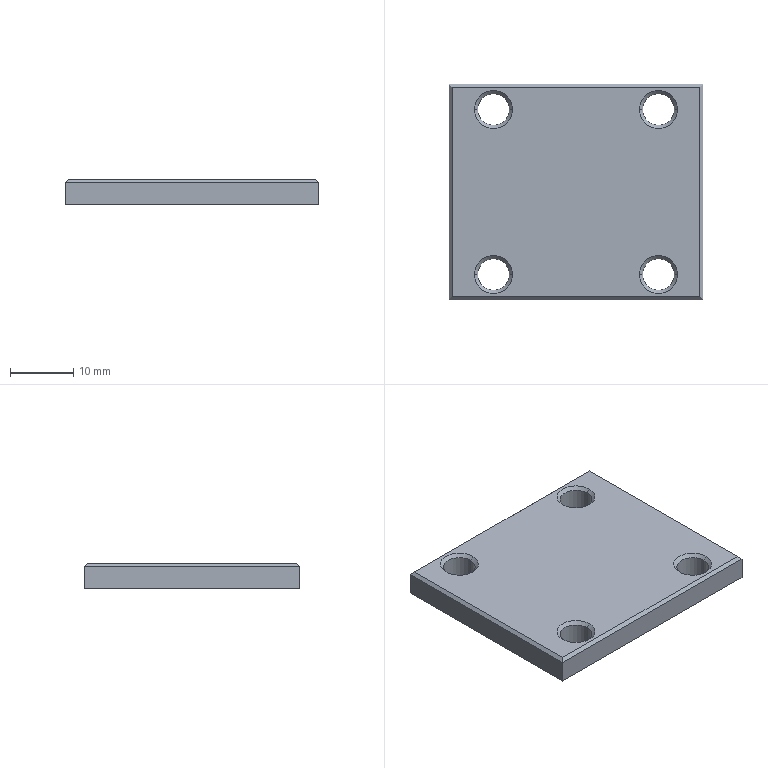Part | NX | 1 solid | 26 faces | box 40 x 34 x 4.05 mm | volume 5163 mm3 | plane 10 | cylinder 8 | cone 8 | commonest cylinder face diameters 5 x8
STEP:
#1=CARTESIAN_POINT('',(0.,0.,8.07));
#2=VERTEX_POINT('',#1);
#3=CARTESIAN_POINT('',(0.,-34.,8.07));
#4=VERTEX_POINT('',#3);
#5=CARTESIAN_POINT('',(0.,0.,8.07));
#6=DIRECTION('',(0.,-1.,0.));
#7=VECTOR('',#6,1000.);
#8=LINE('',#5,#7);
#9=EDGE_CURVE('',#2,#4,#8,.T.);
#10=ORIENTED_EDGE('',*,*,#9,.T.);
#11=CARTESIAN_POINT('',(0.5,-33.5,8.57));
#12=VERTEX_POINT('',#11);
#13=CARTESIAN_POINT('',(-8.07,-42.07,0.));
#14=DIRECTION('',(0.5774,0.5774,0.5774));
#15=VECTOR('',#14,1000.);
#16=LINE('',#13,#15);
#17=EDGE_CURVE('',#4,#12,#16,.T.);
#18=ORIENTED_EDGE('',*,*,#17,.T.);
#19=CARTESIAN_POINT('',(0.5,-0.5,8.57));
#20=VERTEX_POINT('',#19);
#21=CARTESIAN_POINT('',(0.5,0.,8.57));
#22=DIRECTION('',(0.,-1.,0.));
#23=VECTOR('',#22,1000.);
#24=LINE('',#21,#23);
#25=EDGE_CURVE('',#20,#12,#24,.T.);
#26=ORIENTED_EDGE('',*,*,#25,.F.);
#27=CARTESIAN_POINT('',(-8.07,8.07,0.));
#28=DIRECTION('',(0.5774,-0.5774,0.5774));
#29=VECTOR('',#28,1000.);
#30=LINE('',#27,#29);
#31=EDGE_CURVE('',#2,#20,#30,.T.);
#32=ORIENTED_EDGE('',*,*,#31,.F.);
#33=EDGE_LOOP('',(#10,#18,#26,#32));
#34=FACE_BOUND('',#33,.T.);
#35=CARTESIAN_POINT('',(0.25,-17.,8.32));
#36=DIRECTION('',(0.7071,0.,-0.7071));
#37=DIRECTION('',(0.,-1.,0.));
#38=AXIS2_PLACEMENT_3D('',#35,#36,#37);
#39=PLANE('',#38);
#40=ADVANCED_FACE('',(#34),#39,.F.);
#41=ORIENTED_EDGE('',*,*,#9,.F.);
#42=CARTESIAN_POINT('',(0.,0.,4.52));
#43=VERTEX_POINT('',#42);
#44=CARTESIAN_POINT('',(0.,0.,0.));
#45=DIRECTION('',(0.,0.,-1.));
#46=VECTOR('',#45,1000.);
#47=LINE('',#44,#46);
#48=EDGE_CURVE('',#2,#43,#47,.T.);
#49=ORIENTED_EDGE('',*,*,#48,.T.);
#50=CARTESIAN_POINT('',(0.,-34.,4.52));
#51=VERTEX_POINT('',#50);
#52=CARTESIAN_POINT('',(0.,0.,4.52));
#53=DIRECTION('',(0.,-1.,0.));
#54=VECTOR('',#53,1000.);
#55=LINE('',#52,#54);
#56=EDGE_CURVE('',#43,#51,#55,.T.);
#57=ORIENTED_EDGE('',*,*,#56,.T.);
#58=CARTESIAN_POINT('',(0.,-34.,0.));
#59=DIRECTION('',(0.,0.,1.));
#60=VECTOR('',#59,1000.);
#61=LINE('',#58,#60);
#62=EDGE_CURVE('',#51,#4,#61,.T.);
#63=ORIENTED_EDGE('',*,*,#62,.T.);
#64=EDGE_LOOP('',(#41,#49,#57,#63));
#65=FACE_BOUND('',#64,.T.);
#66=CARTESIAN_POINT('',(0.,0.,0.));
#67=DIRECTION('',(-1.,0.,0.));
#68=DIRECTION('',(0.,0.,1.));
#69=AXIS2_PLACEMENT_3D('',#66,#67,#68);
#70=PLANE('',#69);
#71=ADVANCED_FACE('',(#65),#70,.T.);
#72=CARTESIAN_POINT('',(40.,0.,8.07));
#73=VERTEX_POINT('',#72);
#74=CARTESIAN_POINT('',(0.,0.,8.07));
#75=DIRECTION('',(1.,0.,0.));
#76=VECTOR('',#75,1000.);
#77=LINE('',#74,#76);
#78=EDGE_CURVE('',#2,#73,#77,.T.);
#79=ORIENTED_EDGE('',*,*,#78,.T.);
#80=CARTESIAN_POINT('',(40.,0.,4.52));
#81=VERTEX_POINT('',#80);
#82=CARTESIAN_POINT('',(40.,0.,0.));
#83=DIRECTION('',(0.,0.,1.));
#84=VECTOR('',#83,1000.);
#85=LINE('',#82,#84);
#86=EDGE_CURVE('',#81,#73,#85,.T.);
#87=ORIENTED_EDGE('',*,*,#86,.F.);
#88=CARTESIAN_POINT('',(0.,0.,4.52));
#89=DIRECTION('',(-1.,0.,0.));
#90=VECTOR('',#89,1000.);
#91=LINE('',#88,#90);
#92=EDGE_CURVE('',#81,#43,#91,.T.);
#93=ORIENTED_EDGE('',*,*,#92,.T.);
#94=ORIENTED_EDGE('',*,*,#48,.F.);
#95=EDGE_LOOP('',(#79,#87,#93,#94));
#96=FACE_BOUND('',#95,.T.);
#97=CARTESIAN_POINT('',(40.,0.,0.));
#98=DIRECTION('',(0.,1.,0.));
#99=DIRECTION('',(1.,0.,0.));
#100=AXIS2_PLACEMENT_3D('',#97,#98,#99);
#101=PLANE('',#100);
#102=ADVANCED_FACE('',(#96),#101,.T.);
#103=CARTESIAN_POINT('',(40.,-34.,8.07));
#104=VERTEX_POINT('',#103);
#105=CARTESIAN_POINT('',(40.,0.,8.07));
#106=DIRECTION('',(0.,1.,0.));
#107=VECTOR('',#106,1000.);
#108=LINE('',#105,#107);
#109=EDGE_CURVE('',#104,#73,#108,.T.);
#110=ORIENTED_EDGE('',*,*,#109,.F.);
#111=CARTESIAN_POINT('',(40.,-34.,4.52));
#112=VERTEX_POINT('',#111);
#113=CARTESIAN_POINT('',(40.,-34.,0.));
#114=DIRECTION('',(0.,0.,-1.));
#115=VECTOR('',#114,1000.);
#116=LINE('',#113,#115);
#117=EDGE_CURVE('',#104,#112,#116,.T.);
#118=ORIENTED_EDGE('',*,*,#117,.T.);
#119=CARTESIAN_POINT('',(40.,0.,4.52));
#120=DIRECTION('',(0.,1.,0.));
#121=VECTOR('',#120,1000.);
#122=LINE('',#119,#121);
#123=EDGE_CURVE('',#112,#81,#122,.T.);
#124=ORIENTED_EDGE('',*,*,#123,.T.);
#125=ORIENTED_EDGE('',*,*,#86,.T.);
#126=EDGE_LOOP('',(#110,#118,#124,#125));
#127=FACE_BOUND('',#126,.T.);
#128=CARTESIAN_POINT('',(40.,-34.,0.));
#129=DIRECTION('',(1.,0.,0.));
#130=DIRECTION('',(0.,1.,0.));
#131=AXIS2_PLACEMENT_3D('',#128,#129,#130);
#132=PLANE('',#131);
#133=ADVANCED_FACE('',(#127),#132,.T.);
#134=CARTESIAN_POINT('',(0.,-34.,8.07));
#135=DIRECTION('',(1.,0.,0.));
#136=VECTOR('',#135,1000.);
#137=LINE('',#134,#136);
#138=EDGE_CURVE('',#4,#104,#137,.T.);
#139=ORIENTED_EDGE('',*,*,#138,.F.);
#140=ORIENTED_EDGE('',*,*,#62,.F.);
#141=CARTESIAN_POINT('',(0.,-34.,4.52));
#142=DIRECTION('',(1.,0.,0.));
#143=VECTOR('',#142,1000.);
#144=LINE('',#141,#143);
#145=EDGE_CURVE('',#51,#112,#144,.T.);
#146=ORIENTED_EDGE('',*,*,#145,.T.);
#147=ORIENTED_EDGE('',*,*,#117,.F.);
#148=EDGE_LOOP('',(#139,#140,#146,#147));
#149=FACE_BOUND('',#148,.T.);
#150=CARTESIAN_POINT('',(0.,-34.,0.));
#151=DIRECTION('',(0.,-1.,0.));
#152=DIRECTION('',(0.,0.,-1.));
#153=AXIS2_PLACEMENT_3D('',#150,#151,#152);
#154=PLANE('',#153);
#155=ADVANCED_FACE('',(#149),#154,.T.);
#156=ORIENTED_EDGE('',*,*,#92,.F.);
#157=ORIENTED_EDGE('',*,*,#123,.F.);
#158=ORIENTED_EDGE('',*,*,#145,.F.);
#159=ORIENTED_EDGE('',*,*,#56,.F.);
#160=EDGE_LOOP('',(#156,#157,#158,#159));
#161=FACE_BOUND('',#160,.T.);
#162=CARTESIAN_POINT('',(4.5,-30.,4.52));
#163=VERTEX_POINT('',#162);
#164=CARTESIAN_POINT('',(9.5,-30.,4.52));
#165=VERTEX_POINT('',#164);
#166=CARTESIAN_POINT('',(7.,-30.,4.52));
#167=DIRECTION('',(0.,0.,-1.));
#168=DIRECTION('',(-1.,0.,0.));
#169=AXIS2_PLACEMENT_3D('',#166,#167,#168);
#170=CIRCLE('',#169,2.5);
#171=EDGE_CURVE('',#163,#165,#170,.T.);
#172=ORIENTED_EDGE('',*,*,#171,.F.);
#173=CARTESIAN_POINT('',(7.,-30.,4.52));
#174=DIRECTION('',(0.,0.,-1.));
#175=DIRECTION('',(-1.,0.,0.));
#176=AXIS2_PLACEMENT_3D('',#173,#174,#175);
#177=CIRCLE('',#176,2.5);
#178=EDGE_CURVE('',#165,#163,#177,.T.);
#179=ORIENTED_EDGE('',*,*,#178,.F.);
#180=EDGE_LOOP('',(#172,#179));
#181=FACE_BOUND('',#180,.T.);
#182=CARTESIAN_POINT('',(4.5,-4.,4.52));
#183=VERTEX_POINT('',#182);
#184=CARTESIAN_POINT('',(9.5,-4.,4.52));
#185=VERTEX_POINT('',#184);
#186=CARTESIAN_POINT('',(7.,-4.,4.52));
#187=DIRECTION('',(0.,0.,-1.));
#188=DIRECTION('',(-1.,0.,0.));
#189=AXIS2_PLACEMENT_3D('',#186,#187,#188);
#190=CIRCLE('',#189,2.5);
#191=EDGE_CURVE('',#183,#185,#190,.T.);
#192=ORIENTED_EDGE('',*,*,#191,.F.);
#193=CARTESIAN_POINT('',(7.,-4.,4.52));
#194=DIRECTION('',(0.,0.,-1.));
#195=DIRECTION('',(-1.,0.,0.));
#196=AXIS2_PLACEMENT_3D('',#193,#194,#195);
#197=CIRCLE('',#196,2.5);
#198=EDGE_CURVE('',#185,#183,#197,.T.);
#199=ORIENTED_EDGE('',*,*,#198,.F.);
#200=EDGE_LOOP('',(#192,#199));
#201=FACE_BOUND('',#200,.T.);
#202=CARTESIAN_POINT('',(30.5,-4.,4.52));
#203=VERTEX_POINT('',#202);
#204=CARTESIAN_POINT('',(35.5,-4.,4.52));
#205=VERTEX_POINT('',#204);
#206=CARTESIAN_POINT('',(33.,-4.,4.52));
#207=DIRECTION('',(0.,0.,-1.));
#208=DIRECTION('',(-1.,0.,0.));
#209=AXIS2_PLACEMENT_3D('',#206,#207,#208);
#210=CIRCLE('',#209,2.5);
#211=EDGE_CURVE('',#203,#205,#210,.T.);
#212=ORIENTED_EDGE('',*,*,#211,.F.);
#213=CARTESIAN_POINT('',(33.,-4.,4.52));
#214=DIRECTION('',(0.,0.,-1.));
#215=DIRECTION('',(-1.,0.,0.));
#216=AXIS2_PLACEMENT_3D('',#213,#214,#215);
#217=CIRCLE('',#216,2.5);
#218=EDGE_CURVE('',#205,#203,#217,.T.);
#219=ORIENTED_EDGE('',*,*,#218,.F.);
#220=EDGE_LOOP('',(#212,#219));
#221=FACE_BOUND('',#220,.T.);
#222=CARTESIAN_POINT('',(30.5,-30.,4.52));
#223=VERTEX_POINT('',#222);
#224=CARTESIAN_POINT('',(35.5,-30.,4.52));
#225=VERTEX_POINT('',#224);
#226=CARTESIAN_POINT('',(33.,-30.,4.52));
#227=DIRECTION('',(0.,0.,-1.));
#228=DIRECTION('',(-1.,0.,0.));
#229=AXIS2_PLACEMENT_3D('',#226,#227,#228);
#230=CIRCLE('',#229,2.5);
#231=EDGE_CURVE('',#223,#225,#230,.T.);
#232=ORIENTED_EDGE('',*,*,#231,.F.);
#233=CARTESIAN_POINT('',(33.,-30.,4.52));
#234=DIRECTION('',(0.,0.,-1.));
#235=DIRECTION('',(-1.,0.,0.));
#236=AXIS2_PLACEMENT_3D('',#233,#234,#235);
#237=CIRCLE('',#236,2.5);
#238=EDGE_CURVE('',#225,#223,#237,.T.);
#239=ORIENTED_EDGE('',*,*,#238,.F.);
#240=EDGE_LOOP('',(#232,#239));
#241=FACE_BOUND('',#240,.T.);
#242=CARTESIAN_POINT('',(-167.,62.,4.52));
#243=DIRECTION('',(0.,0.,1.));
#244=DIRECTION('',(1.,0.,0.));
#245=AXIS2_PLACEMENT_3D('',#242,#243,#244);
#246=PLANE('',#245);
#247=ADVANCED_FACE('',(#161,#181,#201,#221,#241),#246,.F.);
#248=CARTESIAN_POINT('',(9.5,-4.,8.07));
#249=VERTEX_POINT('',#248);
#250=CARTESIAN_POINT('',(4.5,-4.,8.07));
#251=VERTEX_POINT('',#250);
#252=CARTESIAN_POINT('',(7.,-4.,8.07));
#253=DIRECTION('',(0.,0.,-1.));
#254=DIRECTION('',(-1.,0.,0.));
#255=AXIS2_PLACEMENT_3D('',#252,#253,#254);
#256=CIRCLE('',#255,2.5);
#257=EDGE_CURVE('',#249,#251,#256,.T.);
#258=ORIENTED_EDGE('',*,*,#257,.F.);
#259=CARTESIAN_POINT('',(9.5,-4.,10.5));
#260=DIRECTION('',(0.,0.,-1.));
#261=VECTOR('',#260,1000.);
#262=LINE('',#259,#261);
#263=EDGE_CURVE('',#249,#185,#262,.T.);
#264=ORIENTED_EDGE('',*,*,#263,.T.);
#265=ORIENTED_EDGE('',*,*,#198,.T.);
#266=CARTESIAN_POINT('',(4.5,-4.,10.5));
#267=DIRECTION('',(0.,0.,-1.));
#268=VECTOR('',#267,1000.);
#269=LINE('',#266,#268);
#270=EDGE_CURVE('',#251,#183,#269,.T.);
#271=ORIENTED_EDGE('',*,*,#270,.F.);
#272=EDGE_LOOP('',(#258,#264,#265,#271));
#273=FACE_BOUND('',#272,.T.);
#274=CARTESIAN_POINT('',(7.,-4.,10.5));
#275=DIRECTION('',(0.,0.,-1.));
#276=DIRECTION('',(-1.,0.,0.));
#277=AXIS2_PLACEMENT_3D('',#274,#275,#276);
#278=CYLINDRICAL_SURFACE('',#277,2.5);
#279=ADVANCED_FACE('',(#273),#278,.F.);
#280=CARTESIAN_POINT('',(35.5,-4.,8.07));
#281=VERTEX_POINT('',#280);
#282=CARTESIAN_POINT('',(30.5,-4.,8.07));
#283=VERTEX_POINT('',#282);
#284=CARTESIAN_POINT('',(33.,-4.,8.07));
#285=DIRECTION('',(0.,0.,1.));
#286=DIRECTION('',(1.,0.,0.));
#287=AXIS2_PLACEMENT_3D('',#284,#285,#286);
#288=CIRCLE('',#287,2.5);
#289=EDGE_CURVE('',#281,#283,#288,.T.);
#290=ORIENTED_EDGE('',*,*,#289,.T.);
#291=CARTESIAN_POINT('',(30.5,-4.,10.5));
#292=DIRECTION('',(0.,0.,-1.));
#293=VECTOR('',#292,1000.);
#294=LINE('',#291,#293);
#295=EDGE_CURVE('',#203,#283,#294,.F.);
#296=ORIENTED_EDGE('',*,*,#295,.F.);
#297=ORIENTED_EDGE('',*,*,#211,.T.);
#298=CARTESIAN_POINT('',(35.5,-4.,10.5));
#299=DIRECTION('',(0.,0.,-1.));
#300=VECTOR('',#299,1000.);
#301=LINE('',#298,#300);
#302=EDGE_CURVE('',#205,#281,#301,.F.);
#303=ORIENTED_EDGE('',*,*,#302,.T.);
#304=EDGE_LOOP('',(#290,#296,#297,#303));
#305=FACE_BOUND('',#304,.T.);
#306=CARTESIAN_POINT('',(33.,-4.,10.5));
#307=DIRECTION('',(0.,0.,-1.));
#308=DIRECTION('',(-1.,0.,0.));
#309=AXIS2_PLACEMENT_3D('',#306,#307,#308);
#310=CYLINDRICAL_SURFACE('',#309,2.5);
#311=ADVANCED_FACE('',(#305),#310,.F.);
#312=ORIENTED_EDGE('',*,*,#171,.T.);
#313=CARTESIAN_POINT('',(9.5,-30.,8.07));
#314=VERTEX_POINT('',#313);
#315=CARTESIAN_POINT('',(9.5,-30.,10.5));
#316=DIRECTION('',(0.,0.,-1.));
#317=VECTOR('',#316,1000.);
#318=LINE('',#315,#317);
#319=EDGE_CURVE('',#314,#165,#318,.T.);
#320=ORIENTED_EDGE('',*,*,#319,.F.);
#321=CARTESIAN_POINT('',(4.5,-30.,8.07));
#322=VERTEX_POINT('',#321);
#323=CARTESIAN_POINT('',(7.,-30.,8.07));
#324=DIRECTION('',(0.,0.,1.));
#325=DIRECTION('',(1.,0.,0.));
#326=AXIS2_PLACEMENT_3D('',#323,#324,#325);
#327=CIRCLE('',#326,2.5);
#328=EDGE_CURVE('',#314,#322,#327,.T.);
#329=ORIENTED_EDGE('',*,*,#328,.T.);
#330=CARTESIAN_POINT('',(4.5,-30.,10.5));
#331=DIRECTION('',(0.,0.,-1.));
#332=VECTOR('',#331,1000.);
#333=LINE('',#330,#332);
#334=EDGE_CURVE('',#322,#163,#333,.T.);
#335=ORIENTED_EDGE('',*,*,#334,.T.);
#336=EDGE_LOOP('',(#312,#320,#329,#335));
#337=FACE_BOUND('',#336,.T.);
#338=CARTESIAN_POINT('',(7.,-30.,10.5));
#339=DIRECTION('',(0.,0.,-1.));
#340=DIRECTION('',(-1.,0.,0.));
#341=AXIS2_PLACEMENT_3D('',#338,#339,#340);
#342=CYLINDRICAL_SURFACE('',#341,2.5);
#343=ADVANCED_FACE('',(#337),#342,.F.);
#344=ORIENTED_EDGE('',*,*,#231,.T.);
#345=CARTESIAN_POINT('',(35.5,-30.,8.07));
#346=VERTEX_POINT('',#345);
#347=CARTESIAN_POINT('',(35.5,-30.,10.5));
#348=DIRECTION('',(0.,0.,-1.));
#349=VECTOR('',#348,1000.);
#350=LINE('',#347,#349);
#351=EDGE_CURVE('',#346,#225,#350,.T.);
#352=ORIENTED_EDGE('',*,*,#351,.F.);
#353=CARTESIAN_POINT('',(30.5,-30.,8.07));
#354=VERTEX_POINT('',#353);
#355=CARTESIAN_POINT('',(33.,-30.,8.07));
#356=DIRECTION('',(0.,0.,-1.));
#357=DIRECTION('',(-1.,0.,0.));
#358=AXIS2_PLACEMENT_3D('',#355,#356,#357);
#359=CIRCLE('',#358,2.5);
#360=EDGE_CURVE('',#354,#346,#359,.T.);
#361=ORIENTED_EDGE('',*,*,#360,.F.);
#362=CARTESIAN_POINT('',(30.5,-30.,10.5));
#363=DIRECTION('',(0.,0.,-1.));
#364=VECTOR('',#363,1000.);
#365=LINE('',#362,#364);
#366=EDGE_CURVE('',#354,#223,#365,.T.);
#367=ORIENTED_EDGE('',*,*,#366,.T.);
#368=EDGE_LOOP('',(#344,#352,#361,#367));
#369=FACE_BOUND('',#368,.T.);
#370=CARTESIAN_POINT('',(33.,-30.,10.5));
#371=DIRECTION('',(0.,0.,-1.));
#372=DIRECTION('',(-1.,0.,0.));
#373=AXIS2_PLACEMENT_3D('',#370,#371,#372);
#374=CYLINDRICAL_SURFACE('',#373,2.5);
#375=ADVANCED_FACE('',(#369),#374,.F.);
#376=ORIENTED_EDGE('',*,*,#257,.T.);
#377=CARTESIAN_POINT('',(4.,-4.,8.57));
#378=VERTEX_POINT('',#377);
#379=CARTESIAN_POINT('',(4.,-4.,8.57));
#380=DIRECTION('',(-0.7071,0.,0.7071));
#381=VECTOR('',#380,1000.);
#382=LINE('',#379,#381);
#383=EDGE_CURVE('',#378,#251,#382,.F.);
#384=ORIENTED_EDGE('',*,*,#383,.F.);
#385=CARTESIAN_POINT('',(10.,-4.,8.57));
#386=VERTEX_POINT('',#385);
#387=CARTESIAN_POINT('',(7.,-4.,8.57));
#388=DIRECTION('',(0.,0.,1.));
#389=DIRECTION('',(1.,0.,0.));
#390=AXIS2_PLACEMENT_3D('',#387,#388,#389);
#391=CIRCLE('',#390,3.);
#392=EDGE_CURVE('',#378,#386,#391,.T.);
#393=ORIENTED_EDGE('',*,*,#392,.T.);
#394=CARTESIAN_POINT('',(10.,-4.,8.57));
#395=DIRECTION('',(0.7071,0.,0.7071));
#396=VECTOR('',#395,1000.);
#397=LINE('',#394,#396);
#398=EDGE_CURVE('',#386,#249,#397,.F.);
#399=ORIENTED_EDGE('',*,*,#398,.T.);
#400=EDGE_LOOP('',(#376,#384,#393,#399));
#401=FACE_BOUND('',#400,.T.);
#402=CARTESIAN_POINT('',(7.,-4.,8.57));
#403=DIRECTION('',(0.,0.,1.));
#404=DIRECTION('',(1.,0.,0.));
#405=AXIS2_PLACEMENT_3D('',#402,#403,#404);
#406=CONICAL_SURFACE('',#405,3.,0.7854);
#407=ADVANCED_FACE('',(#401),#406,.F.);
#408=CARTESIAN_POINT('',(7.,-30.,8.07));
#409=DIRECTION('',(0.,0.,1.));
#410=DIRECTION('',(1.,0.,0.));
#411=AXIS2_PLACEMENT_3D('',#408,#409,#410);
#412=CIRCLE('',#411,2.5);
#413=EDGE_CURVE('',#322,#314,#412,.T.);
#414=ORIENTED_EDGE('',*,*,#413,.F.);
#415=CARTESIAN_POINT('',(4.,-30.,8.57));
#416=VERTEX_POINT('',#415);
#417=CARTESIAN_POINT('',(4.,-30.,8.57));
#418=DIRECTION('',(-0.7071,0.,0.7071));
#419=VECTOR('',#418,1000.);
#420=LINE('',#417,#419);
#421=EDGE_CURVE('',#322,#416,#420,.T.);
#422=ORIENTED_EDGE('',*,*,#421,.T.);
#423=CARTESIAN_POINT('',(10.,-30.,8.57));
#424=VERTEX_POINT('',#423);
#425=CARTESIAN_POINT('',(7.,-30.,8.57));
#426=DIRECTION('',(0.,0.,1.));
#427=DIRECTION('',(1.,0.,0.));
#428=AXIS2_PLACEMENT_3D('',#425,#426,#427);
#429=CIRCLE('',#428,3.);
#430=EDGE_CURVE('',#416,#424,#429,.T.);
#431=ORIENTED_EDGE('',*,*,#430,.T.);
#432=CARTESIAN_POINT('',(10.,-30.,8.57));
#433=DIRECTION('',(0.7071,0.,0.7071));
#434=VECTOR('',#433,1000.);
#435=LINE('',#432,#434);
#436=EDGE_CURVE('',#314,#424,#435,.T.);
#437=ORIENTED_EDGE('',*,*,#436,.F.);
#438=EDGE_LOOP('',(#414,#422,#431,#437));
#439=FACE_BOUND('',#438,.T.);
#440=CARTESIAN_POINT('',(7.,-30.,8.57));
#441=DIRECTION('',(0.,0.,1.));
#442=DIRECTION('',(1.,0.,0.));
#443=AXIS2_PLACEMENT_3D('',#440,#441,#442);
#444=CONICAL_SURFACE('',#443,3.,0.7854);
#445=ADVANCED_FACE('',(#439),#444,.F.);
#446=CARTESIAN_POINT('',(30.,-30.,8.57));
#447=VERTEX_POINT('',#446);
#448=CARTESIAN_POINT('',(36.,-30.,8.57));
#449=VERTEX_POINT('',#448);
#450=CARTESIAN_POINT('',(33.,-30.,8.57));
#451=DIRECTION('',(0.,0.,1.));
#452=DIRECTION('',(1.,0.,0.));
#453=AXIS2_PLACEMENT_3D('',#450,#451,#452);
#454=CIRCLE('',#453,3.);
#455=EDGE_CURVE('',#447,#449,#454,.T.);
#456=ORIENTED_EDGE('',*,*,#455,.T.);
#457=CARTESIAN_POINT('',(36.,-30.,8.57));
#458=DIRECTION('',(0.7071,0.,0.7071));
#459=VECTOR('',#458,1000.);
#460=LINE('',#457,#459);
#461=EDGE_CURVE('',#346,#449,#460,.T.);
#462=ORIENTED_EDGE('',*,*,#461,.F.);
#463=CARTESIAN_POINT('',(33.,-30.,8.07));
#464=DIRECTION('',(0.,0.,-1.));
#465=DIRECTION('',(-1.,0.,0.));
#466=AXIS2_PLACEMENT_3D('',#463,#464,#465);
#467=CIRCLE('',#466,2.5);
#468=EDGE_CURVE('',#346,#354,#467,.T.);
#469=ORIENTED_EDGE('',*,*,#468,.T.);
#470=CARTESIAN_POINT('',(30.,-30.,8.57));
#471=DIRECTION('',(-0.7071,0.,0.7071));
#472=VECTOR('',#471,1000.);
#473=LINE('',#470,#472);
#474=EDGE_CURVE('',#354,#447,#473,.T.);
#475=ORIENTED_EDGE('',*,*,#474,.T.);
#476=EDGE_LOOP('',(#456,#462,#469,#475));
#477=FACE_BOUND('',#476,.T.);
#478=CARTESIAN_POINT('',(33.,-30.,8.57));
#479=DIRECTION('',(0.,0.,1.));
#480=DIRECTION('',(1.,0.,0.));
#481=AXIS2_PLACEMENT_3D('',#478,#479,#480);
#482=CONICAL_SURFACE('',#481,3.,0.7854);
#483=ADVANCED_FACE('',(#477),#482,.F.);
#484=CARTESIAN_POINT('',(36.,-4.,8.57));
#485=VERTEX_POINT('',#484);
#486=CARTESIAN_POINT('',(30.,-4.,8.57));
#487=VERTEX_POINT('',#486);
#488=CARTESIAN_POINT('',(33.,-4.,8.57));
#489=DIRECTION('',(0.,0.,1.));
#490=DIRECTION('',(1.,0.,0.));
#491=AXIS2_PLACEMENT_3D('',#488,#489,#490);
#492=CIRCLE('',#491,3.);
#493=EDGE_CURVE('',#485,#487,#492,.T.);
#494=ORIENTED_EDGE('',*,*,#493,.T.);
#495=CARTESIAN_POINT('',(30.,-4.,8.57));
#496=DIRECTION('',(-0.7071,0.,0.7071));
#497=VECTOR('',#496,1000.);
#498=LINE('',#495,#497);
#499=EDGE_CURVE('',#283,#487,#498,.T.);
#500=ORIENTED_EDGE('',*,*,#499,.F.);
#501=ORIENTED_EDGE('',*,*,#289,.F.);
#502=CARTESIAN_POINT('',(36.,-4.,8.57));
#503=DIRECTION('',(0.7071,0.,0.7071));
#504=VECTOR('',#503,1000.);
#505=LINE('',#502,#504);
#506=EDGE_CURVE('',#281,#485,#505,.T.);
#507=ORIENTED_EDGE('',*,*,#506,.T.);
#508=EDGE_LOOP('',(#494,#500,#501,#507));
#509=FACE_BOUND('',#508,.T.);
#510=CARTESIAN_POINT('',(33.,-4.,8.57));
#511=DIRECTION('',(0.,0.,1.));
#512=DIRECTION('',(1.,0.,0.));
#513=AXIS2_PLACEMENT_3D('',#510,#511,#512);
#514=CONICAL_SURFACE('',#513,3.,0.7854);
#515=ADVANCED_FACE('',(#509),#514,.F.);
#516=ORIENTED_EDGE('',*,*,#138,.T.);
#517=CARTESIAN_POINT('',(39.5,-33.5,8.57));
#518=VERTEX_POINT('',#517);
#519=CARTESIAN_POINT('',(48.07,-42.07,0.));
#520=DIRECTION('',(-0.5774,0.5774,0.5774));
#521=VECTOR('',#520,1000.);
#522=LINE('',#519,#521);
#523=EDGE_CURVE('',#104,#518,#522,.T.);
#524=ORIENTED_EDGE('',*,*,#523,.T.);
#525=CARTESIAN_POINT('',(0.,-33.5,8.57));
#526=DIRECTION('',(1.,0.,0.));
#527=VECTOR('',#526,1000.);
#528=LINE('',#525,#527);
#529=EDGE_CURVE('',#12,#518,#528,.T.);
#530=ORIENTED_EDGE('',*,*,#529,.F.);
#531=ORIENTED_EDGE('',*,*,#17,.F.);
#532=EDGE_LOOP('',(#516,#524,#530,#531));
#533=FACE_BOUND('',#532,.T.);
#534=CARTESIAN_POINT('',(20.,-33.75,8.32));
#535=DIRECTION('',(0.,0.7071,-0.7071));
#536=DIRECTION('',(-1.,0.,0.));
#537=AXIS2_PLACEMENT_3D('',#534,#535,#536);
#538=PLANE('',#537);
#539=ADVANCED_FACE('',(#533),#538,.F.);
#540=ORIENTED_EDGE('',*,*,#109,.T.);
#541=CARTESIAN_POINT('',(39.5,-0.5,8.57));
#542=VERTEX_POINT('',#541);
#543=CARTESIAN_POINT('',(48.07,8.07,0.));
#544=DIRECTION('',(-0.5774,-0.5774,0.5774));
#545=VECTOR('',#544,1000.);
#546=LINE('',#543,#545);
#547=EDGE_CURVE('',#73,#542,#546,.T.);
#548=ORIENTED_EDGE('',*,*,#547,.T.);
#549=CARTESIAN_POINT('',(39.5,0.,8.57));
#550=DIRECTION('',(0.,-1.,0.));
#551=VECTOR('',#550,1000.);
#552=LINE('',#549,#551);
#553=EDGE_CURVE('',#542,#518,#552,.T.);
#554=ORIENTED_EDGE('',*,*,#553,.T.);
#555=ORIENTED_EDGE('',*,*,#523,.F.);
#556=EDGE_LOOP('',(#540,#548,#554,#555));
#557=FACE_BOUND('',#556,.T.);
#558=CARTESIAN_POINT('',(39.75,-17.,8.32));
#559=DIRECTION('',(0.7071,0.,0.7071));
#560=DIRECTION('',(0.,-1.,0.));
#561=AXIS2_PLACEMENT_3D('',#558,#559,#560);
#562=PLANE('',#561);
#563=ADVANCED_FACE('',(#557),#562,.T.);
#564=ORIENTED_EDGE('',*,*,#78,.F.);
#565=ORIENTED_EDGE('',*,*,#31,.T.);
#566=CARTESIAN_POINT('',(0.,-0.5,8.57));
#567=DIRECTION('',(1.,0.,0.));
#568=VECTOR('',#567,1000.);
#569=LINE('',#566,#568);
#570=EDGE_CURVE('',#20,#542,#569,.T.);
#571=ORIENTED_EDGE('',*,*,#570,.T.);
#572=ORIENTED_EDGE('',*,*,#547,.F.);
#573=EDGE_LOOP('',(#564,#565,#571,#572));
#574=FACE_BOUND('',#573,.T.);
#575=CARTESIAN_POINT('',(20.,-0.25,8.32));
#576=DIRECTION('',(0.,0.7071,0.7071));
#577=DIRECTION('',(1.,0.,0.));
#578=AXIS2_PLACEMENT_3D('',#575,#576,#577);
#579=PLANE('',#578);
#580=ADVANCED_FACE('',(#574),#579,.T.);
#581=ORIENTED_EDGE('',*,*,#25,.T.);
#582=ORIENTED_EDGE('',*,*,#529,.T.);
#583=ORIENTED_EDGE('',*,*,#553,.F.);
#584=ORIENTED_EDGE('',*,*,#570,.F.);
#585=EDGE_LOOP('',(#581,#582,#583,#584));
#586=FACE_BOUND('',#585,.T.);
#587=CARTESIAN_POINT('',(7.,-4.,8.57));
#588=DIRECTION('',(0.,0.,1.));
#589=DIRECTION('',(1.,0.,0.));
#590=AXIS2_PLACEMENT_3D('',#587,#588,#589);
#591=CIRCLE('',#590,3.);
#592=EDGE_CURVE('',#386,#378,#591,.T.);
#593=ORIENTED_EDGE('',*,*,#592,.F.);
#594=ORIENTED_EDGE('',*,*,#392,.F.);
#595=EDGE_LOOP('',(#593,#594));
#596=FACE_BOUND('',#595,.T.);
#597=ORIENTED_EDGE('',*,*,#455,.F.);
#598=CARTESIAN_POINT('',(33.,-30.,8.57));
#599=DIRECTION('',(0.,0.,1.));
#600=DIRECTION('',(1.,0.,0.));
#601=AXIS2_PLACEMENT_3D('',#598,#599,#600);
#602=CIRCLE('',#601,3.);
#603=EDGE_CURVE('',#449,#447,#602,.T.);
#604=ORIENTED_EDGE('',*,*,#603,.F.);
#605=EDGE_LOOP('',(#597,#604));
#606=FACE_BOUND('',#605,.T.);
#607=ORIENTED_EDGE('',*,*,#493,.F.);
#608=CARTESIAN_POINT('',(33.,-4.,8.57));
#609=DIRECTION('',(0.,0.,1.));
#610=DIRECTION('',(1.,0.,0.));
#611=AXIS2_PLACEMENT_3D('',#608,#609,#610);
#612=CIRCLE('',#611,3.);
#613=EDGE_CURVE('',#487,#485,#612,.T.);
#614=ORIENTED_EDGE('',*,*,#613,.F.);
#615=EDGE_LOOP('',(#607,#614));
#616=FACE_BOUND('',#615,.T.);
#617=ORIENTED_EDGE('',*,*,#430,.F.);
#618=CARTESIAN_POINT('',(7.,-30.,8.57));
#619=DIRECTION('',(0.,0.,1.));
#620=DIRECTION('',(1.,0.,0.));
#621=AXIS2_PLACEMENT_3D('',#618,#619,#620);
#622=CIRCLE('',#621,3.);
#623=EDGE_CURVE('',#424,#416,#622,.T.);
#624=ORIENTED_EDGE('',*,*,#623,.F.);
#625=EDGE_LOOP('',(#617,#624));
#626=FACE_BOUND('',#625,.T.);
#627=CARTESIAN_POINT('',(0.,0.,8.57));
#628=DIRECTION('',(0.,0.,1.));
#629=DIRECTION('',(1.,0.,0.));
#630=AXIS2_PLACEMENT_3D('',#627,#628,#629);
#631=PLANE('',#630);
#632=ADVANCED_FACE('',(#586,#596,#606,#616,#626),#631,.T.);
#633=ORIENTED_EDGE('',*,*,#461,.T.);
#634=ORIENTED_EDGE('',*,*,#603,.T.);
#635=ORIENTED_EDGE('',*,*,#474,.F.);
#636=ORIENTED_EDGE('',*,*,#360,.T.);
#637=EDGE_LOOP('',(#633,#634,#635,#636));
#638=FACE_BOUND('',#637,.T.);
#639=CARTESIAN_POINT('',(33.,-30.,8.57));
#640=DIRECTION('',(0.,0.,1.));
#641=DIRECTION('',(1.,0.,0.));
#642=AXIS2_PLACEMENT_3D('',#639,#640,#641);
#643=CONICAL_SURFACE('',#642,3.,0.7854);
#644=ADVANCED_FACE('',(#638),#643,.F.);
#645=ORIENTED_EDGE('',*,*,#295,.T.);
#646=CARTESIAN_POINT('',(33.,-4.,8.07));
#647=DIRECTION('',(0.,0.,1.));
#648=DIRECTION('',(1.,0.,0.));
#649=AXIS2_PLACEMENT_3D('',#646,#647,#648);
#650=CIRCLE('',#649,2.5);
#651=EDGE_CURVE('',#283,#281,#650,.T.);
#652=ORIENTED_EDGE('',*,*,#651,.T.);
#653=ORIENTED_EDGE('',*,*,#302,.F.);
#654=ORIENTED_EDGE('',*,*,#218,.T.);
#655=EDGE_LOOP('',(#645,#652,#653,#654));
#656=FACE_BOUND('',#655,.T.);
#657=CARTESIAN_POINT('',(33.,-4.,10.5));
#658=DIRECTION('',(0.,0.,-1.));
#659=DIRECTION('',(-1.,0.,0.));
#660=AXIS2_PLACEMENT_3D('',#657,#658,#659);
#661=CYLINDRICAL_SURFACE('',#660,2.5);
#662=ADVANCED_FACE('',(#656),#661,.F.);
#663=ORIENTED_EDGE('',*,*,#506,.F.);
#664=ORIENTED_EDGE('',*,*,#651,.F.);
#665=ORIENTED_EDGE('',*,*,#499,.T.);
#666=ORIENTED_EDGE('',*,*,#613,.T.);
#667=EDGE_LOOP('',(#663,#664,#665,#666));
#668=FACE_BOUND('',#667,.T.);
#669=CARTESIAN_POINT('',(33.,-4.,8.57));
#670=DIRECTION('',(0.,0.,1.));
#671=DIRECTION('',(1.,0.,0.));
#672=AXIS2_PLACEMENT_3D('',#669,#670,#671);
#673=CONICAL_SURFACE('',#672,3.,0.7854);
#674=ADVANCED_FACE('',(#668),#673,.F.);
#675=ORIENTED_EDGE('',*,*,#413,.T.);
#676=ORIENTED_EDGE('',*,*,#319,.T.);
#677=ORIENTED_EDGE('',*,*,#178,.T.);
#678=ORIENTED_EDGE('',*,*,#334,.F.);
#679=EDGE_LOOP('',(#675,#676,#677,#678));
#680=FACE_BOUND('',#679,.T.);
#681=CARTESIAN_POINT('',(7.,-30.,10.5));
#682=DIRECTION('',(0.,0.,-1.));
#683=DIRECTION('',(-1.,0.,0.));
#684=AXIS2_PLACEMENT_3D('',#681,#682,#683);
#685=CYLINDRICAL_SURFACE('',#684,2.5);
#686=ADVANCED_FACE('',(#680),#685,.F.);
#687=ORIENTED_EDGE('',*,*,#592,.T.);
#688=ORIENTED_EDGE('',*,*,#383,.T.);
#689=CARTESIAN_POINT('',(7.,-4.,8.07));
#690=DIRECTION('',(0.,0.,-1.));
#691=DIRECTION('',(-1.,0.,0.));
#692=AXIS2_PLACEMENT_3D('',#689,#690,#691);
#693=CIRCLE('',#692,2.5);
#694=EDGE_CURVE('',#251,#249,#693,.T.);
#695=ORIENTED_EDGE('',*,*,#694,.T.);
#696=ORIENTED_EDGE('',*,*,#398,.F.);
#697=EDGE_LOOP('',(#687,#688,#695,#696));
#698=FACE_BOUND('',#697,.T.);
#699=CARTESIAN_POINT('',(7.,-4.,8.57));
#700=DIRECTION('',(0.,0.,1.));
#701=DIRECTION('',(1.,0.,0.));
#702=AXIS2_PLACEMENT_3D('',#699,#700,#701);
#703=CONICAL_SURFACE('',#702,3.,0.7854);
#704=ADVANCED_FACE('',(#698),#703,.F.);
#705=ORIENTED_EDGE('',*,*,#468,.F.);
#706=ORIENTED_EDGE('',*,*,#351,.T.);
#707=ORIENTED_EDGE('',*,*,#238,.T.);
#708=ORIENTED_EDGE('',*,*,#366,.F.);
#709=EDGE_LOOP('',(#705,#706,#707,#708));
#710=FACE_BOUND('',#709,.T.);
#711=CARTESIAN_POINT('',(33.,-30.,10.5));
#712=DIRECTION('',(0.,0.,-1.));
#713=DIRECTION('',(-1.,0.,0.));
#714=AXIS2_PLACEMENT_3D('',#711,#712,#713);
#715=CYLINDRICAL_SURFACE('',#714,2.5);
#716=ADVANCED_FACE('',(#710),#715,.F.);
#717=ORIENTED_EDGE('',*,*,#436,.T.);
#718=ORIENTED_EDGE('',*,*,#623,.T.);
#719=ORIENTED_EDGE('',*,*,#421,.F.);
#720=ORIENTED_EDGE('',*,*,#328,.F.);
#721=EDGE_LOOP('',(#717,#718,#719,#720));
#722=FACE_BOUND('',#721,.T.);
#723=CARTESIAN_POINT('',(7.,-30.,8.57));
#724=DIRECTION('',(0.,0.,1.));
#725=DIRECTION('',(1.,0.,0.));
#726=AXIS2_PLACEMENT_3D('',#723,#724,#725);
#727=CONICAL_SURFACE('',#726,3.,0.7854);
#728=ADVANCED_FACE('',(#722),#727,.F.);
#729=ORIENTED_EDGE('',*,*,#191,.T.);
#730=ORIENTED_EDGE('',*,*,#263,.F.);
#731=ORIENTED_EDGE('',*,*,#694,.F.);
#732=ORIENTED_EDGE('',*,*,#270,.T.);
#733=EDGE_LOOP('',(#729,#730,#731,#732));
#734=FACE_BOUND('',#733,.T.);
#735=CARTESIAN_POINT('',(7.,-4.,10.5));
#736=DIRECTION('',(0.,0.,-1.));
#737=DIRECTION('',(-1.,0.,0.));
#738=AXIS2_PLACEMENT_3D('',#735,#736,#737);
#739=CYLINDRICAL_SURFACE('',#738,2.5);
#740=ADVANCED_FACE('',(#734),#739,.F.);
#741=CLOSED_SHELL('',(#40,#71,#102,#133,#155,#247,#279,#311,#343,#375,#407,#445,#483,#515,#539,#563,#580,#632,#644,#662,#674,#686,#704,#716,#728,#740));
#742=MANIFOLD_SOLID_BREP('',#741);
#743=(LENGTH_UNIT()NAMED_UNIT(*)SI_UNIT(.MILLI.,.METRE.));
#744=UNCERTAINTY_MEASURE_WITH_UNIT(LENGTH_MEASURE(0.00001),#743,'','');
#745=(NAMED_UNIT(*)PLANE_ANGLE_UNIT()SI_UNIT($,.RADIAN.));
#746=(NAMED_UNIT(*)SI_UNIT($,.STERADIAN.)SOLID_ANGLE_UNIT());
#747=(GEOMETRIC_REPRESENTATION_CONTEXT(3)GLOBAL_UNCERTAINTY_ASSIGNED_CONTEXT((#744))GLOBAL_UNIT_ASSIGNED_CONTEXT((#743,#745,#746))REPRESENTATION_CONTEXT('',''));
#748=ADVANCED_BREP_SHAPE_REPRESENTATION('',(#742),#747);